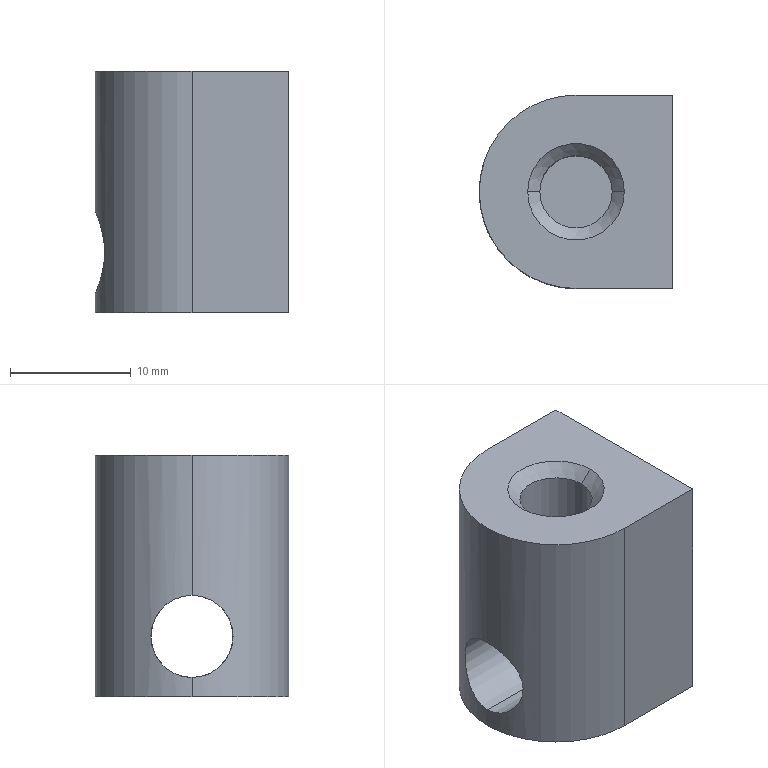Part | 1 solid | 14 faces | box 16 x 16 x 20 mm | volume 3703 mm3 | cylinder 6 | plane 6 | cone 2 | commonest cylinder face diameters 6 x2 6.8 x2 16 x2
STEP:
#1=CARTESIAN_POINT('',(-3.,0.,9.));
#2=VERTEX_POINT('',#1);
#3=CARTESIAN_POINT('',(3.,0.,9.));
#4=VERTEX_POINT('',#3);
#5=CARTESIAN_POINT('',(0.,0.,9.));
#6=DIRECTION('',(0.,0.,1.));
#7=DIRECTION('',(1.,0.,0.));
#8=AXIS2_PLACEMENT_3D('',#5,#6,#7);
#9=CIRCLE('',#8,3.);
#10=EDGE_CURVE('',#2,#4,#9,.T.);
#11=ORIENTED_EDGE('',*,*,#10,.F.);
#12=CARTESIAN_POINT('',(-4.,0.,10.));
#13=VERTEX_POINT('',#12);
#14=CARTESIAN_POINT('',(-3.,0.,9.));
#15=DIRECTION('',(-0.7071,0.,0.7071));
#16=VECTOR('',#15,1000.);
#17=LINE('',#14,#16);
#18=EDGE_CURVE('',#2,#13,#17,.T.);
#19=ORIENTED_EDGE('',*,*,#18,.T.);
#20=CARTESIAN_POINT('',(4.,0.,10.));
#21=VERTEX_POINT('',#20);
#22=CARTESIAN_POINT('',(0.,0.,10.));
#23=DIRECTION('',(0.,0.,-1.));
#24=DIRECTION('',(1.,0.,0.));
#25=AXIS2_PLACEMENT_3D('',#22,#23,#24);
#26=CIRCLE('',#25,4.);
#27=EDGE_CURVE('',#21,#13,#26,.T.);
#28=ORIENTED_EDGE('',*,*,#27,.F.);
#29=CARTESIAN_POINT('',(3.,0.,9.));
#30=DIRECTION('',(0.7071,0.,0.7071));
#31=VECTOR('',#30,1000.);
#32=LINE('',#29,#31);
#33=EDGE_CURVE('',#4,#21,#32,.T.);
#34=ORIENTED_EDGE('',*,*,#33,.F.);
#35=EDGE_LOOP('',(#11,#19,#28,#34));
#36=FACE_OUTER_BOUND('',#35,.T.);
#37=CARTESIAN_POINT('',(0.,0.,9.));
#38=DIRECTION('',(0.,0.,1.));
#39=DIRECTION('',(1.,0.,0.));
#40=AXIS2_PLACEMENT_3D('',#37,#38,#39);
#41=CONICAL_SURFACE('',#40,3.,0.7854);
#42=ADVANCED_FACE('',(#36),#41,.F.);
#43=CARTESIAN_POINT('',(-8.,0.,-1.6));
#44=VERTEX_POINT('',#43);
#45=CARTESIAN_POINT('',(-8.,0.,-8.4));
#46=VERTEX_POINT('',#45);
#47=CARTESIAN_POINT('',(-8.,0.,-1.6));
#48=CARTESIAN_POINT('',(-8.,-0.224,-1.6));
#49=CARTESIAN_POINT('',(-7.99,-0.4515,-1.623));
#50=CARTESIAN_POINT('',(-7.953,-0.8919,-1.711));
#51=CARTESIAN_POINT('',(-7.926,-1.105,-1.777));
#52=CARTESIAN_POINT('',(-7.858,-1.517,-1.949));
#53=CARTESIAN_POINT('',(-7.816,-1.714,-2.055));
#54=CARTESIAN_POINT('',(-7.727,-2.079,-2.301));
#55=CARTESIAN_POINT('',(-7.679,-2.25,-2.442));
#56=CARTESIAN_POINT('',(-7.58,-2.562,-2.754));
#57=CARTESIAN_POINT('',(-7.531,-2.701,-2.924));
#58=CARTESIAN_POINT('',(-7.439,-2.946,-3.288));
#59=CARTESIAN_POINT('',(-7.395,-3.053,-3.486));
#60=CARTESIAN_POINT('',(-7.322,-3.223,-3.896));
#61=CARTESIAN_POINT('',(-7.293,-3.288,-4.108));
#62=CARTESIAN_POINT('',(-7.252,-3.377,-4.547));
#63=CARTESIAN_POINT('',(-7.242,-3.4,-4.775));
#64=CARTESIAN_POINT('',(-7.242,-3.4,-5.223));
#65=CARTESIAN_POINT('',(-7.252,-3.378,-5.446));
#66=CARTESIAN_POINT('',(-7.293,-3.289,-5.891));
#67=CARTESIAN_POINT('',(-7.322,-3.224,-6.104));
#68=CARTESIAN_POINT('',(-7.395,-3.053,-6.513));
#69=CARTESIAN_POINT('',(-7.439,-2.946,-6.711));
#70=CARTESIAN_POINT('',(-7.531,-2.701,-7.077));
#71=CARTESIAN_POINT('',(-7.581,-2.562,-7.247));
#72=CARTESIAN_POINT('',(-7.679,-2.25,-7.559));
#73=CARTESIAN_POINT('',(-7.728,-2.078,-7.7));
#74=CARTESIAN_POINT('',(-7.817,-1.714,-7.945));
#75=CARTESIAN_POINT('',(-7.857,-1.518,-8.05));
#76=CARTESIAN_POINT('',(-7.926,-1.104,-8.223));
#77=CARTESIAN_POINT('',(-7.953,-0.8916,-8.289));
#78=CARTESIAN_POINT('',(-7.99,-0.4541,-8.377));
#79=CARTESIAN_POINT('',(-8.,-0.2274,-8.4));
#80=CARTESIAN_POINT('',(-8.,0.,-8.4));
#81=B_SPLINE_CURVE_WITH_KNOTS('',3,(#47,#48,#49,#50,#51,#52,#53,#54,#55,#56,#57,#58,#59,#60,#61,#62,#63,#64,#65,#66,#67,#68,#69,#70,#71,#72,#73,#74,#75,#76,#77,#78,#79,#80),.UNSPECIFIED.,.F.,.F.,(4,2,2,2,2,2,2,2,2,2,2,2,2,2,2,2,4),(0.01076,0.01143,0.0121,0.01278,0.01345,0.01412,0.01479,0.01546,0.01613,0.01681,0.01748,0.01815,0.01882,0.01949,0.02017,0.02084,0.02151),.UNSPECIFIED.);
#82=EDGE_CURVE('',#44,#46,#81,.T.);
#83=ORIENTED_EDGE('',*,*,#82,.F.);
#84=CARTESIAN_POINT('',(8.,0.,-1.6));
#85=VERTEX_POINT('',#84);
#86=CARTESIAN_POINT('',(8.,0.,-1.6));
#87=DIRECTION('',(1.,0.,0.));
#88=VECTOR('',#87,1000.);
#89=LINE('',#86,#88);
#90=EDGE_CURVE('',#44,#85,#89,.T.);
#91=ORIENTED_EDGE('',*,*,#90,.T.);
#92=CARTESIAN_POINT('',(8.,0.,-8.4));
#93=VERTEX_POINT('',#92);
#94=CARTESIAN_POINT('',(8.,0.,-5.));
#95=DIRECTION('',(1.,0.,0.));
#96=DIRECTION('',(0.,0.,-1.));
#97=AXIS2_PLACEMENT_3D('',#94,#95,#96);
#98=CIRCLE('',#97,3.4);
#99=EDGE_CURVE('',#85,#93,#98,.T.);
#100=ORIENTED_EDGE('',*,*,#99,.T.);
#101=CARTESIAN_POINT('',(8.,0.,-8.4));
#102=DIRECTION('',(1.,0.,0.));
#103=VECTOR('',#102,1000.);
#104=LINE('',#101,#103);
#105=EDGE_CURVE('',#46,#93,#104,.T.);
#106=ORIENTED_EDGE('',*,*,#105,.F.);
#107=EDGE_LOOP('',(#83,#91,#100,#106));
#108=FACE_OUTER_BOUND('',#107,.T.);
#109=CARTESIAN_POINT('',(8.,0.,-5.));
#110=DIRECTION('',(1.,0.,0.));
#111=DIRECTION('',(0.,0.,-1.));
#112=AXIS2_PLACEMENT_3D('',#109,#110,#111);
#113=CYLINDRICAL_SURFACE('',#112,3.4);
#114=ADVANCED_FACE('',(#108),#113,.F.);
#115=CARTESIAN_POINT('',(-3.,0.,0.));
#116=VERTEX_POINT('',#115);
#117=CARTESIAN_POINT('',(3.,0.,0.));
#118=VERTEX_POINT('',#117);
#119=CARTESIAN_POINT('',(0.,0.,0.));
#120=DIRECTION('',(0.,0.,1.));
#121=DIRECTION('',(1.,0.,0.));
#122=AXIS2_PLACEMENT_3D('',#119,#120,#121);
#123=CIRCLE('',#122,3.);
#124=EDGE_CURVE('',#116,#118,#123,.T.);
#125=ORIENTED_EDGE('',*,*,#124,.F.);
#126=CARTESIAN_POINT('',(-3.,0.,0.));
#127=DIRECTION('',(0.,0.,1.));
#128=VECTOR('',#127,1000.);
#129=LINE('',#126,#128);
#130=EDGE_CURVE('',#116,#2,#129,.T.);
#131=ORIENTED_EDGE('',*,*,#130,.T.);
#132=ORIENTED_EDGE('',*,*,#10,.T.);
#133=CARTESIAN_POINT('',(3.,0.,0.));
#134=DIRECTION('',(0.,0.,1.));
#135=VECTOR('',#134,1000.);
#136=LINE('',#133,#135);
#137=EDGE_CURVE('',#118,#4,#136,.T.);
#138=ORIENTED_EDGE('',*,*,#137,.F.);
#139=EDGE_LOOP('',(#125,#131,#132,#138));
#140=FACE_OUTER_BOUND('',#139,.T.);
#141=CARTESIAN_POINT('',(0.,0.,0.));
#142=DIRECTION('',(0.,0.,1.));
#143=DIRECTION('',(1.,0.,0.));
#144=AXIS2_PLACEMENT_3D('',#141,#142,#143);
#145=CYLINDRICAL_SURFACE('',#144,3.);
#146=ADVANCED_FACE('',(#140),#145,.F.);
#147=CARTESIAN_POINT('',(-8.,0.,10.));
#148=VERTEX_POINT('',#147);
#149=CARTESIAN_POINT('',(0.,-8.,10.));
#150=VERTEX_POINT('',#149);
#151=CARTESIAN_POINT('',(0.,0.,10.));
#152=DIRECTION('',(0.,0.,1.));
#153=DIRECTION('',(1.,0.,0.));
#154=AXIS2_PLACEMENT_3D('',#151,#152,#153);
#155=CIRCLE('',#154,8.);
#156=EDGE_CURVE('',#148,#150,#155,.T.);
#157=ORIENTED_EDGE('',*,*,#156,.F.);
#158=CARTESIAN_POINT('',(-8.,0.,10.));
#159=DIRECTION('',(0.,0.,-1.));
#160=VECTOR('',#159,1000.);
#161=LINE('',#158,#160);
#162=EDGE_CURVE('',#148,#44,#161,.T.);
#163=ORIENTED_EDGE('',*,*,#162,.T.);
#164=ORIENTED_EDGE('',*,*,#82,.T.);
#165=CARTESIAN_POINT('',(-8.,0.,-10.));
#166=VERTEX_POINT('',#165);
#167=CARTESIAN_POINT('',(-8.,0.,10.));
#168=DIRECTION('',(0.,0.,-1.));
#169=VECTOR('',#168,1000.);
#170=LINE('',#167,#169);
#171=EDGE_CURVE('',#46,#166,#170,.T.);
#172=ORIENTED_EDGE('',*,*,#171,.T.);
#173=CARTESIAN_POINT('',(0.,-8.,-10.));
#174=VERTEX_POINT('',#173);
#175=CARTESIAN_POINT('',(0.,0.,-10.));
#176=DIRECTION('',(0.,0.,1.));
#177=DIRECTION('',(1.,0.,0.));
#178=AXIS2_PLACEMENT_3D('',#175,#176,#177);
#179=CIRCLE('',#178,8.);
#180=EDGE_CURVE('',#166,#174,#179,.T.);
#181=ORIENTED_EDGE('',*,*,#180,.T.);
#182=CARTESIAN_POINT('',(0.,-8.,10.));
#183=DIRECTION('',(0.,0.,-1.));
#184=VECTOR('',#183,1000.);
#185=LINE('',#182,#184);
#186=EDGE_CURVE('',#150,#174,#185,.T.);
#187=ORIENTED_EDGE('',*,*,#186,.F.);
#188=EDGE_LOOP('',(#157,#163,#164,#172,#181,#187));
#189=FACE_OUTER_BOUND('',#188,.T.);
#190=CARTESIAN_POINT('',(0.,0.,10.));
#191=DIRECTION('',(0.,0.,-1.));
#192=DIRECTION('',(-1.,0.,0.));
#193=AXIS2_PLACEMENT_3D('',#190,#191,#192);
#194=CYLINDRICAL_SURFACE('',#193,8.);
#195=ADVANCED_FACE('',(#189),#194,.T.);
#196=ORIENTED_EDGE('',*,*,#162,.F.);
#197=CARTESIAN_POINT('',(0.,8.,10.));
#198=VERTEX_POINT('',#197);
#199=CARTESIAN_POINT('',(0.,0.,10.));
#200=DIRECTION('',(0.,0.,1.));
#201=DIRECTION('',(1.,0.,0.));
#202=AXIS2_PLACEMENT_3D('',#199,#200,#201);
#203=CIRCLE('',#202,8.);
#204=EDGE_CURVE('',#198,#148,#203,.T.);
#205=ORIENTED_EDGE('',*,*,#204,.F.);
#206=CARTESIAN_POINT('',(0.,8.,-10.));
#207=VERTEX_POINT('',#206);
#208=CARTESIAN_POINT('',(0.,8.,10.));
#209=DIRECTION('',(0.,0.,-1.));
#210=VECTOR('',#209,1000.);
#211=LINE('',#208,#210);
#212=EDGE_CURVE('',#198,#207,#211,.T.);
#213=ORIENTED_EDGE('',*,*,#212,.T.);
#214=CARTESIAN_POINT('',(0.,0.,-10.));
#215=DIRECTION('',(0.,0.,1.));
#216=DIRECTION('',(1.,0.,0.));
#217=AXIS2_PLACEMENT_3D('',#214,#215,#216);
#218=CIRCLE('',#217,8.);
#219=EDGE_CURVE('',#207,#166,#218,.T.);
#220=ORIENTED_EDGE('',*,*,#219,.T.);
#221=ORIENTED_EDGE('',*,*,#171,.F.);
#222=CARTESIAN_POINT('',(-8.,0.,-8.4));
#223=CARTESIAN_POINT('',(-8.,0.2276,-8.4));
#224=CARTESIAN_POINT('',(-7.99,0.4508,-8.377));
#225=CARTESIAN_POINT('',(-7.953,0.8892,-8.289));
#226=CARTESIAN_POINT('',(-7.926,1.107,-8.223));
#227=CARTESIAN_POINT('',(-7.858,1.517,-8.051));
#228=CARTESIAN_POINT('',(-7.817,1.712,-7.946));
#229=CARTESIAN_POINT('',(-7.727,2.08,-7.699));
#230=CARTESIAN_POINT('',(-7.678,2.251,-7.557));
#231=CARTESIAN_POINT('',(-7.581,2.561,-7.247));
#232=CARTESIAN_POINT('',(-7.531,2.701,-7.077));
#233=CARTESIAN_POINT('',(-7.438,2.948,-6.708));
#234=CARTESIAN_POINT('',(-7.395,3.052,-6.514));
#235=CARTESIAN_POINT('',(-7.323,3.222,-6.107));
#236=CARTESIAN_POINT('',(-7.293,3.289,-5.89));
#237=CARTESIAN_POINT('',(-7.252,3.378,-5.45));
#238=CARTESIAN_POINT('',(-7.242,3.4,-5.227));
#239=CARTESIAN_POINT('',(-7.241,3.4,-4.777));
#240=CARTESIAN_POINT('',(-7.252,3.377,-4.549));
#241=CARTESIAN_POINT('',(-7.293,3.289,-4.111));
#242=CARTESIAN_POINT('',(-7.322,3.224,-3.896));
#243=CARTESIAN_POINT('',(-7.396,3.051,-3.483));
#244=CARTESIAN_POINT('',(-7.439,2.946,-3.289));
#245=CARTESIAN_POINT('',(-7.531,2.701,-2.923));
#246=CARTESIAN_POINT('',(-7.582,2.559,-2.75));
#247=CARTESIAN_POINT('',(-7.679,2.248,-2.44));
#248=CARTESIAN_POINT('',(-7.727,2.079,-2.301));
#249=CARTESIAN_POINT('',(-7.817,1.711,-2.054));
#250=CARTESIAN_POINT('',(-7.858,1.514,-1.948));
#251=CARTESIAN_POINT('',(-7.926,1.105,-1.777));
#252=CARTESIAN_POINT('',(-7.953,0.8924,-1.711));
#253=CARTESIAN_POINT('',(-7.991,0.448,-1.622));
#254=CARTESIAN_POINT('',(-8.,0.2242,-1.6));
#255=CARTESIAN_POINT('',(-8.,0.,-1.6));
#256=B_SPLINE_CURVE_WITH_KNOTS('',3,(#222,#223,#224,#225,#226,#227,#228,#229,#230,#231,#232,#233,#234,#235,#236,#237,#238,#239,#240,#241,#242,#243,#244,#245,#246,#247,#248,#249,#250,#251,#252,#253,#254,#255),.UNSPECIFIED.,.F.,.F.,(4,2,2,2,2,2,2,2,2,2,2,2,2,2,2,2,4),(0.,0.0006725,0.001345,0.002017,0.00269,0.003362,0.004035,0.004707,0.00538,0.006052,0.006725,0.007397,0.00807,0.008742,0.009415,0.01009,0.01076),.UNSPECIFIED.);
#257=EDGE_CURVE('',#46,#44,#256,.T.);
#258=ORIENTED_EDGE('',*,*,#257,.T.);
#259=EDGE_LOOP('',(#196,#205,#213,#220,#221,#258));
#260=FACE_OUTER_BOUND('',#259,.T.);
#261=CARTESIAN_POINT('',(0.,0.,10.));
#262=DIRECTION('',(0.,0.,-1.));
#263=DIRECTION('',(-1.,0.,0.));
#264=AXIS2_PLACEMENT_3D('',#261,#262,#263);
#265=CYLINDRICAL_SURFACE('',#264,8.);
#266=ADVANCED_FACE('',(#260),#265,.T.);
#267=CARTESIAN_POINT('',(8.,-8.,-10.));
#268=VERTEX_POINT('',#267);
#269=CARTESIAN_POINT('',(0.,-8.,-10.));
#270=DIRECTION('',(1.,0.,0.));
#271=VECTOR('',#270,1000.);
#272=LINE('',#269,#271);
#273=EDGE_CURVE('',#174,#268,#272,.T.);
#274=ORIENTED_EDGE('',*,*,#273,.T.);
#275=CARTESIAN_POINT('',(8.,-8.,10.));
#276=VERTEX_POINT('',#275);
#277=CARTESIAN_POINT('',(8.,-8.,10.));
#278=DIRECTION('',(0.,0.,-1.));
#279=VECTOR('',#278,1000.);
#280=LINE('',#277,#279);
#281=EDGE_CURVE('',#276,#268,#280,.T.);
#282=ORIENTED_EDGE('',*,*,#281,.F.);
#283=CARTESIAN_POINT('',(0.,-8.,10.));
#284=DIRECTION('',(1.,0.,0.));
#285=VECTOR('',#284,1000.);
#286=LINE('',#283,#285);
#287=EDGE_CURVE('',#150,#276,#286,.T.);
#288=ORIENTED_EDGE('',*,*,#287,.F.);
#289=ORIENTED_EDGE('',*,*,#186,.T.);
#290=EDGE_LOOP('',(#274,#282,#288,#289));
#291=FACE_OUTER_BOUND('',#290,.T.);
#292=CARTESIAN_POINT('',(0.,-8.,10.));
#293=DIRECTION('',(0.,1.,0.));
#294=DIRECTION('',(0.,0.,1.));
#295=AXIS2_PLACEMENT_3D('',#292,#293,#294);
#296=PLANE('',#295);
#297=ADVANCED_FACE('',(#291),#296,.F.);
#298=CARTESIAN_POINT('',(8.,0.,-5.));
#299=DIRECTION('',(1.,0.,0.));
#300=DIRECTION('',(0.,0.,-1.));
#301=AXIS2_PLACEMENT_3D('',#298,#299,#300);
#302=CIRCLE('',#301,3.4);
#303=EDGE_CURVE('',#93,#85,#302,.T.);
#304=ORIENTED_EDGE('',*,*,#303,.F.);
#305=ORIENTED_EDGE('',*,*,#99,.F.);
#306=EDGE_LOOP('',(#304,#305));
#307=FACE_BOUND('',#306,.T.);
#308=CARTESIAN_POINT('',(8.,8.,-10.));
#309=VERTEX_POINT('',#308);
#310=CARTESIAN_POINT('',(8.,0.,-10.));
#311=DIRECTION('',(0.,1.,0.));
#312=VECTOR('',#311,1000.);
#313=LINE('',#310,#312);
#314=EDGE_CURVE('',#268,#309,#313,.T.);
#315=ORIENTED_EDGE('',*,*,#314,.T.);
#316=CARTESIAN_POINT('',(8.,8.,10.));
#317=VERTEX_POINT('',#316);
#318=CARTESIAN_POINT('',(8.,8.,10.));
#319=DIRECTION('',(0.,0.,-1.));
#320=VECTOR('',#319,1000.);
#321=LINE('',#318,#320);
#322=EDGE_CURVE('',#317,#309,#321,.T.);
#323=ORIENTED_EDGE('',*,*,#322,.F.);
#324=CARTESIAN_POINT('',(8.,-8.,10.));
#325=DIRECTION('',(0.,1.,0.));
#326=VECTOR('',#325,1000.);
#327=LINE('',#324,#326);
#328=EDGE_CURVE('',#276,#317,#327,.T.);
#329=ORIENTED_EDGE('',*,*,#328,.F.);
#330=ORIENTED_EDGE('',*,*,#281,.T.);
#331=EDGE_LOOP('',(#315,#323,#329,#330));
#332=FACE_OUTER_BOUND('',#331,.T.);
#333=CARTESIAN_POINT('',(8.,0.,10.));
#334=DIRECTION('',(-1.,0.,0.));
#335=DIRECTION('',(0.,0.,1.));
#336=AXIS2_PLACEMENT_3D('',#333,#334,#335);
#337=PLANE('',#336);
#338=ADVANCED_FACE('',(#307,#332),#337,.F.);
#339=CARTESIAN_POINT('',(0.,8.,-10.));
#340=DIRECTION('',(-1.,0.,0.));
#341=VECTOR('',#340,1000.);
#342=LINE('',#339,#341);
#343=EDGE_CURVE('',#309,#207,#342,.T.);
#344=ORIENTED_EDGE('',*,*,#343,.T.);
#345=ORIENTED_EDGE('',*,*,#212,.F.);
#346=CARTESIAN_POINT('',(0.,8.,10.));
#347=DIRECTION('',(-1.,0.,0.));
#348=VECTOR('',#347,1000.);
#349=LINE('',#346,#348);
#350=EDGE_CURVE('',#317,#198,#349,.T.);
#351=ORIENTED_EDGE('',*,*,#350,.F.);
#352=ORIENTED_EDGE('',*,*,#322,.T.);
#353=EDGE_LOOP('',(#344,#345,#351,#352));
#354=FACE_OUTER_BOUND('',#353,.T.);
#355=CARTESIAN_POINT('',(0.,8.,10.));
#356=DIRECTION('',(0.,-1.,0.));
#357=DIRECTION('',(0.,0.,-1.));
#358=AXIS2_PLACEMENT_3D('',#355,#356,#357);
#359=PLANE('',#358);
#360=ADVANCED_FACE('',(#354),#359,.F.);
#361=ORIENTED_EDGE('',*,*,#27,.T.);
#362=CARTESIAN_POINT('',(0.,0.,10.));
#363=DIRECTION('',(0.,0.,-1.));
#364=DIRECTION('',(1.,0.,0.));
#365=AXIS2_PLACEMENT_3D('',#362,#363,#364);
#366=CIRCLE('',#365,4.);
#367=EDGE_CURVE('',#13,#21,#366,.T.);
#368=ORIENTED_EDGE('',*,*,#367,.T.);
#369=EDGE_LOOP('',(#361,#368));
#370=FACE_BOUND('',#369,.T.);
#371=ORIENTED_EDGE('',*,*,#204,.T.);
#372=ORIENTED_EDGE('',*,*,#156,.T.);
#373=ORIENTED_EDGE('',*,*,#287,.T.);
#374=ORIENTED_EDGE('',*,*,#328,.T.);
#375=ORIENTED_EDGE('',*,*,#350,.T.);
#376=EDGE_LOOP('',(#371,#372,#373,#374,#375));
#377=FACE_OUTER_BOUND('',#376,.T.);
#378=CARTESIAN_POINT('',(0.,0.,10.));
#379=DIRECTION('',(0.,0.,1.));
#380=DIRECTION('',(1.,0.,0.));
#381=AXIS2_PLACEMENT_3D('',#378,#379,#380);
#382=PLANE('',#381);
#383=ADVANCED_FACE('',(#370,#377),#382,.T.);
#384=ORIENTED_EDGE('',*,*,#219,.F.);
#385=ORIENTED_EDGE('',*,*,#343,.F.);
#386=ORIENTED_EDGE('',*,*,#314,.F.);
#387=ORIENTED_EDGE('',*,*,#273,.F.);
#388=ORIENTED_EDGE('',*,*,#180,.F.);
#389=EDGE_LOOP('',(#384,#385,#386,#387,#388));
#390=FACE_OUTER_BOUND('',#389,.T.);
#391=CARTESIAN_POINT('',(0.,0.,-10.));
#392=DIRECTION('',(0.,0.,1.));
#393=DIRECTION('',(1.,0.,0.));
#394=AXIS2_PLACEMENT_3D('',#391,#392,#393);
#395=PLANE('',#394);
#396=ADVANCED_FACE('',(#390),#395,.F.);
#397=ORIENTED_EDGE('',*,*,#130,.F.);
#398=CARTESIAN_POINT('',(0.,0.,0.));
#399=DIRECTION('',(0.,0.,1.));
#400=DIRECTION('',(1.,0.,0.));
#401=AXIS2_PLACEMENT_3D('',#398,#399,#400);
#402=CIRCLE('',#401,3.);
#403=EDGE_CURVE('',#118,#116,#402,.T.);
#404=ORIENTED_EDGE('',*,*,#403,.F.);
#405=ORIENTED_EDGE('',*,*,#137,.T.);
#406=CARTESIAN_POINT('',(0.,0.,9.));
#407=DIRECTION('',(0.,0.,1.));
#408=DIRECTION('',(1.,0.,0.));
#409=AXIS2_PLACEMENT_3D('',#406,#407,#408);
#410=CIRCLE('',#409,3.);
#411=EDGE_CURVE('',#4,#2,#410,.T.);
#412=ORIENTED_EDGE('',*,*,#411,.T.);
#413=EDGE_LOOP('',(#397,#404,#405,#412));
#414=FACE_OUTER_BOUND('',#413,.T.);
#415=CARTESIAN_POINT('',(0.,0.,0.));
#416=DIRECTION('',(0.,0.,1.));
#417=DIRECTION('',(1.,0.,0.));
#418=AXIS2_PLACEMENT_3D('',#415,#416,#417);
#419=CYLINDRICAL_SURFACE('',#418,3.);
#420=ADVANCED_FACE('',(#414),#419,.F.);
#421=ORIENTED_EDGE('',*,*,#403,.T.);
#422=ORIENTED_EDGE('',*,*,#124,.T.);
#423=EDGE_LOOP('',(#421,#422));
#424=FACE_OUTER_BOUND('',#423,.T.);
#425=CARTESIAN_POINT('',(0.,0.,0.));
#426=DIRECTION('',(0.,0.,1.));
#427=DIRECTION('',(1.,0.,0.));
#428=AXIS2_PLACEMENT_3D('',#425,#426,#427);
#429=PLANE('',#428);
#430=ADVANCED_FACE('',(#424),#429,.T.);
#431=ORIENTED_EDGE('',*,*,#90,.F.);
#432=ORIENTED_EDGE('',*,*,#257,.F.);
#433=ORIENTED_EDGE('',*,*,#105,.T.);
#434=ORIENTED_EDGE('',*,*,#303,.T.);
#435=EDGE_LOOP('',(#431,#432,#433,#434));
#436=FACE_OUTER_BOUND('',#435,.T.);
#437=CARTESIAN_POINT('',(8.,0.,-5.));
#438=DIRECTION('',(1.,0.,0.));
#439=DIRECTION('',(0.,0.,-1.));
#440=AXIS2_PLACEMENT_3D('',#437,#438,#439);
#441=CYLINDRICAL_SURFACE('',#440,3.4);
#442=ADVANCED_FACE('',(#436),#441,.F.);
#443=ORIENTED_EDGE('',*,*,#18,.F.);
#444=ORIENTED_EDGE('',*,*,#411,.F.);
#445=ORIENTED_EDGE('',*,*,#33,.T.);
#446=ORIENTED_EDGE('',*,*,#367,.F.);
#447=EDGE_LOOP('',(#443,#444,#445,#446));
#448=FACE_OUTER_BOUND('',#447,.T.);
#449=CARTESIAN_POINT('',(0.,0.,9.));
#450=DIRECTION('',(0.,0.,1.));
#451=DIRECTION('',(1.,0.,0.));
#452=AXIS2_PLACEMENT_3D('',#449,#450,#451);
#453=CONICAL_SURFACE('',#452,3.,0.7854);
#454=ADVANCED_FACE('',(#448),#453,.F.);
#455=CLOSED_SHELL('',(#42,#114,#146,#195,#266,#297,#338,#360,#383,#396,#420,#430,#442,#454));
#456=MANIFOLD_SOLID_BREP('',#455);
#457=CARTESIAN_POINT('',(0.,0.,0.));
#458=DIRECTION('',(0.,0.,1.));
#459=DIRECTION('',(1.,0.,0.));
#460=AXIS2_PLACEMENT_3D('',#457,#458,#459);
#461=(LENGTH_UNIT()NAMED_UNIT(*)SI_UNIT(.MILLI.,.METRE.));
#462=UNCERTAINTY_MEASURE_WITH_UNIT(LENGTH_MEASURE(0.00001),#461,'','');
#463=(NAMED_UNIT(*)PLANE_ANGLE_UNIT()SI_UNIT($,.RADIAN.));
#464=(NAMED_UNIT(*)SI_UNIT($,.STERADIAN.)SOLID_ANGLE_UNIT());
#465=(GEOMETRIC_REPRESENTATION_CONTEXT(3)GLOBAL_UNCERTAINTY_ASSIGNED_CONTEXT((#462))GLOBAL_UNIT_ASSIGNED_CONTEXT((#461,#463,#464))REPRESENTATION_CONTEXT('',''));
#466=ADVANCED_BREP_SHAPE_REPRESENTATION('',(#456,#460),#465);